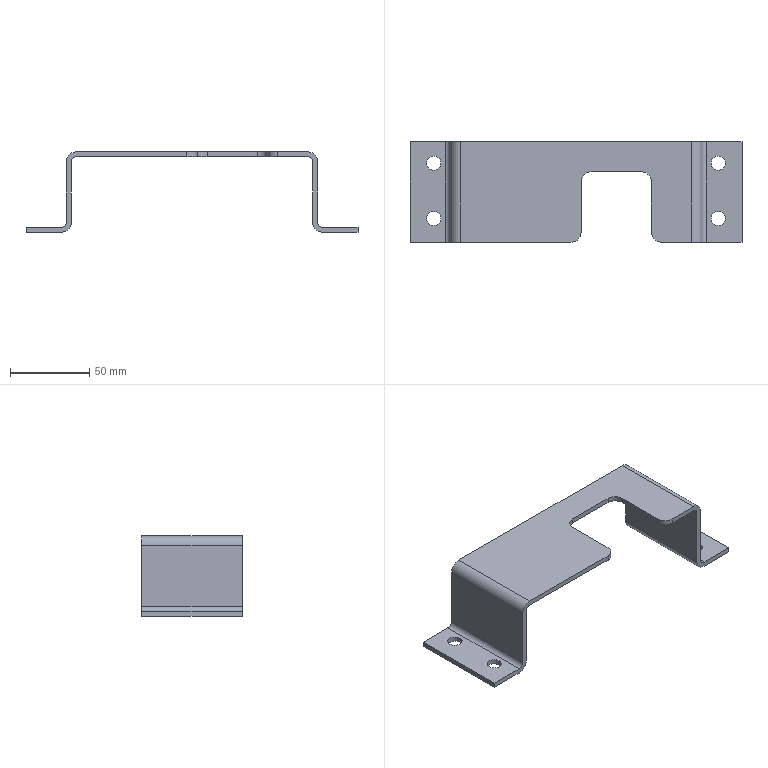Part | STEP file | 1_id1330_x_t | 1 solid | 34 faces | box 209.55 x 63.5 x 50.8 mm | volume 52722 mm3 | plane 18 | cylinder 16 | commonest cylinder face diameters 12.7 x8 6.35 x4 9 x4